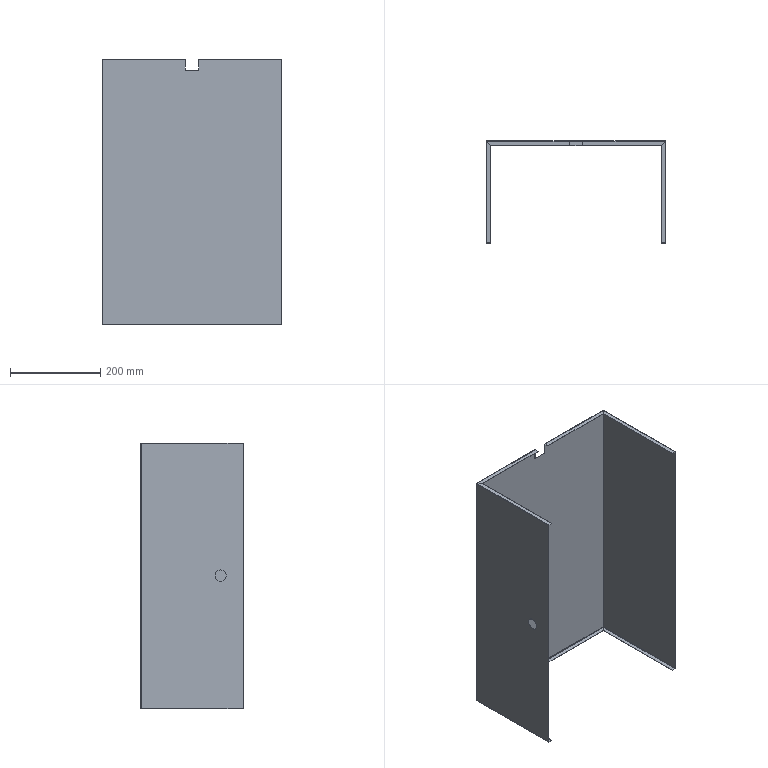Part | SolidWorks | features EdgeFlange 2, ICE 2, FlatPattern 1, SMBaseFlange 1, SheetMetal 1 | 1 solid | 88 faces | box 399.5 x 227 x 590 mm | volume 258240 mm3 | plane 60 | cylinder 20 | spline 8 | commonest cylinder face diameters 0.8 x9 1.8 x9 25 x2